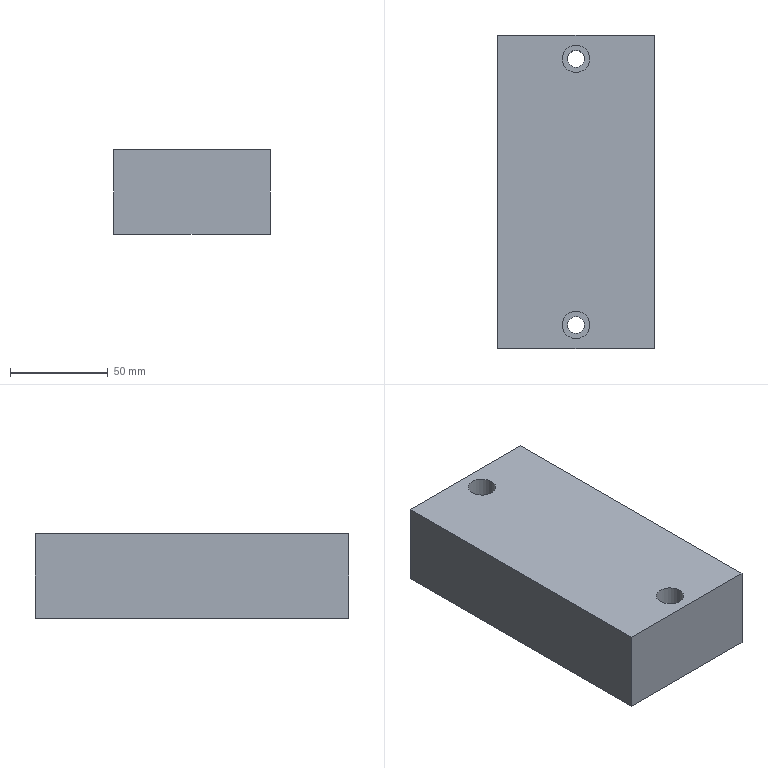Part | STEP file | 200 mesh_id2214 | 1 solid | 18 faces | box 80 x 160 x 43.2 mm | volume 542389 mm3 | plane 8 | cylinder 6 | cone 4 | commonest cylinder face diameters 6.8 x2 8.7 x2 14 x2
STEP:
#1=CARTESIAN_POINT('',(-16566.186,-4088.269,43.2));
#2=VERTEX_POINT('',#1);
#3=CARTESIAN_POINT('',(-16559.186,-4088.269,43.2));
#4=DIRECTION('',(0.,0.,-1.));
#5=DIRECTION('',(-1.,0.,0.));
#6=AXIS2_PLACEMENT_3D('',#3,#4,#5);
#7=CIRCLE('',#6,7.);
#8=EDGE_CURVE('',#2,#2,#7,.T.);
#9=ORIENTED_EDGE('',*,*,#8,.T.);
#10=EDGE_LOOP('',(#9));
#11=FACE_BOUND('',#10,.T.);
#12=CARTESIAN_POINT('',(-16566.186,-3952.269,43.2));
#13=VERTEX_POINT('',#12);
#14=CARTESIAN_POINT('',(-16559.186,-3952.269,43.2));
#15=DIRECTION('',(0.,0.,-1.));
#16=DIRECTION('',(-1.,0.,0.));
#17=AXIS2_PLACEMENT_3D('',#14,#15,#16);
#18=CIRCLE('',#17,7.);
#19=EDGE_CURVE('',#13,#13,#18,.T.);
#20=ORIENTED_EDGE('',*,*,#19,.T.);
#21=EDGE_LOOP('',(#20));
#22=FACE_BOUND('',#21,.T.);
#23=CARTESIAN_POINT('',(-16599.186,-3940.269,43.2));
#24=VERTEX_POINT('',#23);
#25=CARTESIAN_POINT('',(-16519.186,-3940.269,43.2));
#26=VERTEX_POINT('',#25);
#27=CARTESIAN_POINT('',(-16499.186,-3940.269,43.2));
#28=DIRECTION('',(1.,0.,0.));
#29=VECTOR('',#28,1.);
#30=LINE('',#27,#29);
#31=EDGE_CURVE('',#24,#26,#30,.T.);
#32=ORIENTED_EDGE('',*,*,#31,.F.);
#33=CARTESIAN_POINT('',(-16599.186,-4100.269,43.2));
#34=VERTEX_POINT('',#33);
#35=CARTESIAN_POINT('',(-16599.186,-3970.269,43.2));
#36=DIRECTION('',(0.,1.,0.));
#37=VECTOR('',#36,1.);
#38=LINE('',#35,#37);
#39=EDGE_CURVE('',#34,#24,#38,.T.);
#40=ORIENTED_EDGE('',*,*,#39,.F.);
#41=CARTESIAN_POINT('',(-16519.186,-4100.269,43.2));
#42=VERTEX_POINT('',#41);
#43=CARTESIAN_POINT('',(-16599.186,-4100.269,43.2));
#44=DIRECTION('',(-1.,0.,0.));
#45=VECTOR('',#44,1.);
#46=LINE('',#43,#45);
#47=EDGE_CURVE('',#42,#34,#46,.T.);
#48=ORIENTED_EDGE('',*,*,#47,.F.);
#49=CARTESIAN_POINT('',(-16519.186,-4070.269,43.2));
#50=DIRECTION('',(0.,-1.,0.));
#51=VECTOR('',#50,1.);
#52=LINE('',#49,#51);
#53=EDGE_CURVE('',#26,#42,#52,.T.);
#54=ORIENTED_EDGE('',*,*,#53,.F.);
#55=EDGE_LOOP('',(#32,#40,#48,#54));
#56=FACE_BOUND('',#55,.T.);
#57=CARTESIAN_POINT('',(-16648.884,-4140.769,43.2));
#58=DIRECTION('',(0.,0.,1.));
#59=DIRECTION('',(1.,0.,0.));
#60=AXIS2_PLACEMENT_3D('',#57,#58,#59);
#61=PLANE('',#60);
#62=ADVANCED_FACE('',(#11,#22,#56),#61,.T.);
#63=CARTESIAN_POINT('',(-16599.186,-4100.269,0.));
#64=VERTEX_POINT('',#63);
#65=CARTESIAN_POINT('',(-16599.186,-4100.269,0.));
#66=DIRECTION('',(0.,0.,1.));
#67=VECTOR('',#66,1.);
#68=LINE('',#65,#67);
#69=EDGE_CURVE('',#64,#34,#68,.T.);
#70=ORIENTED_EDGE('',*,*,#69,.T.);
#71=ORIENTED_EDGE('',*,*,#39,.T.);
#72=CARTESIAN_POINT('',(-16599.186,-3940.269,0.));
#73=VERTEX_POINT('',#72);
#74=CARTESIAN_POINT('',(-16599.186,-3940.269,0.));
#75=DIRECTION('',(0.,0.,1.));
#76=VECTOR('',#75,1.);
#77=LINE('',#74,#76);
#78=EDGE_CURVE('',#73,#24,#77,.T.);
#79=ORIENTED_EDGE('',*,*,#78,.F.);
#80=CARTESIAN_POINT('',(-16599.186,-3970.269,0.));
#81=DIRECTION('',(0.,-1.,0.));
#82=VECTOR('',#81,1.);
#83=LINE('',#80,#82);
#84=EDGE_CURVE('',#73,#64,#83,.T.);
#85=ORIENTED_EDGE('',*,*,#84,.T.);
#86=EDGE_LOOP('',(#70,#71,#79,#85));
#87=FACE_OUTER_BOUND('',#86,.T.);
#88=CARTESIAN_POINT('',(-16599.186,-3970.269,0.));
#89=DIRECTION('',(-1.,0.,0.));
#90=DIRECTION('',(0.,0.,1.));
#91=AXIS2_PLACEMENT_3D('',#88,#89,#90);
#92=PLANE('',#91);
#93=ADVANCED_FACE('',(#87),#92,.T.);
#94=CARTESIAN_POINT('',(-16554.836,-4088.269,0.));
#95=VERTEX_POINT('',#94);
#96=CARTESIAN_POINT('',(-16559.186,-4088.269,0.));
#97=DIRECTION('',(0.,0.,1.));
#98=DIRECTION('',(1.,0.,0.));
#99=AXIS2_PLACEMENT_3D('',#96,#97,#98);
#100=CIRCLE('',#99,4.35);
#101=EDGE_CURVE('',#95,#95,#100,.T.);
#102=ORIENTED_EDGE('',*,*,#101,.T.);
#103=EDGE_LOOP('',(#102));
#104=FACE_BOUND('',#103,.T.);
#105=CARTESIAN_POINT('',(-16554.836,-3952.269,0.));
#106=VERTEX_POINT('',#105);
#107=CARTESIAN_POINT('',(-16559.186,-3952.269,0.));
#108=DIRECTION('',(0.,0.,1.));
#109=DIRECTION('',(1.,0.,0.));
#110=AXIS2_PLACEMENT_3D('',#107,#108,#109);
#111=CIRCLE('',#110,4.35);
#112=EDGE_CURVE('',#106,#106,#111,.T.);
#113=ORIENTED_EDGE('',*,*,#112,.T.);
#114=EDGE_LOOP('',(#113));
#115=FACE_BOUND('',#114,.T.);
#116=CARTESIAN_POINT('',(-16583.186,-3952.269,0.));
#117=VERTEX_POINT('',#116);
#118=CARTESIAN_POINT('',(-16587.186,-3952.269,0.));
#119=DIRECTION('',(0.,0.,1.));
#120=DIRECTION('',(1.,0.,0.));
#121=AXIS2_PLACEMENT_3D('',#118,#119,#120);
#122=CIRCLE('',#121,4.);
#123=EDGE_CURVE('',#117,#117,#122,.T.);
#124=ORIENTED_EDGE('',*,*,#123,.T.);
#125=EDGE_LOOP('',(#124));
#126=FACE_BOUND('',#125,.T.);
#127=CARTESIAN_POINT('',(-16583.186,-4088.269,0.));
#128=VERTEX_POINT('',#127);
#129=CARTESIAN_POINT('',(-16587.186,-4088.269,0.));
#130=DIRECTION('',(0.,0.,1.));
#131=DIRECTION('',(1.,0.,0.));
#132=AXIS2_PLACEMENT_3D('',#129,#130,#131);
#133=CIRCLE('',#132,4.);
#134=EDGE_CURVE('',#128,#128,#133,.T.);
#135=ORIENTED_EDGE('',*,*,#134,.T.);
#136=EDGE_LOOP('',(#135));
#137=FACE_BOUND('',#136,.T.);
#138=CARTESIAN_POINT('',(-16519.186,-3940.269,0.));
#139=VERTEX_POINT('',#138);
#140=CARTESIAN_POINT('',(2.,-3940.269,0.));
#141=DIRECTION('',(-1.,0.,0.));
#142=VECTOR('',#141,1.);
#143=LINE('',#140,#142);
#144=EDGE_CURVE('',#139,#73,#143,.T.);
#145=ORIENTED_EDGE('',*,*,#144,.F.);
#146=CARTESIAN_POINT('',(-16519.186,-4100.269,0.));
#147=VERTEX_POINT('',#146);
#148=CARTESIAN_POINT('',(-16519.186,0.,0.));
#149=DIRECTION('',(0.,1.,0.));
#150=VECTOR('',#149,1.);
#151=LINE('',#148,#150);
#152=EDGE_CURVE('',#147,#139,#151,.T.);
#153=ORIENTED_EDGE('',*,*,#152,.F.);
#154=CARTESIAN_POINT('',(2.,-4100.269,0.));
#155=DIRECTION('',(1.,0.,0.));
#156=VECTOR('',#155,1.);
#157=LINE('',#154,#156);
#158=EDGE_CURVE('',#64,#147,#157,.T.);
#159=ORIENTED_EDGE('',*,*,#158,.F.);
#160=ORIENTED_EDGE('',*,*,#84,.F.);
#161=EDGE_LOOP('',(#145,#153,#159,#160));
#162=FACE_BOUND('',#161,.T.);
#163=CARTESIAN_POINT('',(2.,0.,0.));
#164=DIRECTION('',(0.,0.,1.));
#165=DIRECTION('',(1.,0.,0.));
#166=AXIS2_PLACEMENT_3D('',#163,#164,#165);
#167=PLANE('',#166);
#168=ADVANCED_FACE('',(#104,#115,#126,#137,#162),#167,.F.);
#169=CARTESIAN_POINT('',(-16519.186,-4100.269,0.));
#170=DIRECTION('',(0.,0.,1.));
#171=VECTOR('',#170,1.);
#172=LINE('',#169,#171);
#173=EDGE_CURVE('',#147,#42,#172,.T.);
#174=ORIENTED_EDGE('',*,*,#173,.T.);
#175=ORIENTED_EDGE('',*,*,#47,.T.);
#176=ORIENTED_EDGE('',*,*,#69,.F.);
#177=ORIENTED_EDGE('',*,*,#158,.T.);
#178=EDGE_LOOP('',(#174,#175,#176,#177));
#179=FACE_OUTER_BOUND('',#178,.T.);
#180=CARTESIAN_POINT('',(-16599.186,-4100.269,0.));
#181=DIRECTION('',(0.,-1.,0.));
#182=DIRECTION('',(0.,0.,-1.));
#183=AXIS2_PLACEMENT_3D('',#180,#181,#182);
#184=PLANE('',#183);
#185=ADVANCED_FACE('',(#179),#184,.T.);
#186=ORIENTED_EDGE('',*,*,#78,.T.);
#187=ORIENTED_EDGE('',*,*,#31,.T.);
#188=CARTESIAN_POINT('',(-16519.186,-3940.269,0.));
#189=DIRECTION('',(0.,0.,1.));
#190=VECTOR('',#189,1.);
#191=LINE('',#188,#190);
#192=EDGE_CURVE('',#139,#26,#191,.T.);
#193=ORIENTED_EDGE('',*,*,#192,.F.);
#194=ORIENTED_EDGE('',*,*,#144,.T.);
#195=EDGE_LOOP('',(#186,#187,#193,#194));
#196=FACE_OUTER_BOUND('',#195,.T.);
#197=CARTESIAN_POINT('',(-16499.186,-3940.269,0.));
#198=DIRECTION('',(0.,1.,0.));
#199=DIRECTION('',(0.,0.,1.));
#200=AXIS2_PLACEMENT_3D('',#197,#198,#199);
#201=PLANE('',#200);
#202=ADVANCED_FACE('',(#196),#201,.T.);
#203=ORIENTED_EDGE('',*,*,#192,.T.);
#204=ORIENTED_EDGE('',*,*,#53,.T.);
#205=ORIENTED_EDGE('',*,*,#173,.F.);
#206=ORIENTED_EDGE('',*,*,#152,.T.);
#207=EDGE_LOOP('',(#203,#204,#205,#206));
#208=FACE_OUTER_BOUND('',#207,.T.);
#209=CARTESIAN_POINT('',(-16519.186,-4070.269,0.));
#210=DIRECTION('',(1.,0.,0.));
#211=DIRECTION('',(0.,0.,-1.));
#212=AXIS2_PLACEMENT_3D('',#209,#210,#211);
#213=PLANE('',#212);
#214=ADVANCED_FACE('',(#208),#213,.T.);
#215=CARTESIAN_POINT('',(-16583.786,-4088.269,35.));
#216=VERTEX_POINT('',#215);
#217=CARTESIAN_POINT('',(-16587.186,-4088.269,35.));
#218=DIRECTION('',(0.,0.,-1.));
#219=DIRECTION('',(1.,0.,0.));
#220=AXIS2_PLACEMENT_3D('',#217,#218,#219);
#221=CIRCLE('',#220,3.4);
#222=EDGE_CURVE('',#216,#216,#221,.T.);
#223=ORIENTED_EDGE('',*,*,#222,.T.);
#224=EDGE_LOOP('',(#223));
#225=FACE_BOUND('',#224,.T.);
#226=CARTESIAN_POINT('',(-16587.186,-4088.269,37.043));
#227=VERTEX_POINT('',#226);
#228=VERTEX_LOOP('',#227);
#229=FACE_BOUND('',#228,.T.);
#230=CARTESIAN_POINT('',(-16587.186,-4088.269,35.));
#231=DIRECTION('',(0.,0.,-1.));
#232=DIRECTION('',(-1.,0.,0.));
#233=AXIS2_PLACEMENT_3D('',#230,#231,#232);
#234=CONICAL_SURFACE('',#233,3.4,59.);
#235=ADVANCED_FACE('',(#225,#229),#234,.F.);
#236=CARTESIAN_POINT('',(-16583.786,-4088.269,0.6));
#237=VERTEX_POINT('',#236);
#238=CARTESIAN_POINT('',(-16587.186,-4088.269,0.6));
#239=DIRECTION('',(0.,0.,-1.));
#240=DIRECTION('',(1.,0.,0.));
#241=AXIS2_PLACEMENT_3D('',#238,#239,#240);
#242=CIRCLE('',#241,3.4);
#243=EDGE_CURVE('',#237,#237,#242,.T.);
#244=ORIENTED_EDGE('',*,*,#243,.T.);
#245=EDGE_LOOP('',(#244));
#246=FACE_BOUND('',#245,.T.);
#247=ORIENTED_EDGE('',*,*,#222,.F.);
#248=EDGE_LOOP('',(#247));
#249=FACE_BOUND('',#248,.T.);
#250=CARTESIAN_POINT('',(-16587.186,-4088.269,0.));
#251=DIRECTION('',(0.,0.,1.));
#252=DIRECTION('',(1.,0.,0.));
#253=AXIS2_PLACEMENT_3D('',#250,#251,#252);
#254=CYLINDRICAL_SURFACE('',#253,3.4);
#255=ADVANCED_FACE('',(#246,#249),#254,.F.);
#256=ORIENTED_EDGE('',*,*,#243,.F.);
#257=EDGE_LOOP('',(#256));
#258=FACE_BOUND('',#257,.T.);
#259=ORIENTED_EDGE('',*,*,#134,.F.);
#260=EDGE_LOOP('',(#259));
#261=FACE_BOUND('',#260,.T.);
#262=CARTESIAN_POINT('',(-16587.186,-4088.269,0.));
#263=DIRECTION('',(0.,0.,-1.));
#264=DIRECTION('',(-1.,0.,0.));
#265=AXIS2_PLACEMENT_3D('',#262,#263,#264);
#266=CONICAL_SURFACE('',#265,4.,45.);
#267=ADVANCED_FACE('',(#258,#261),#266,.F.);
#268=CARTESIAN_POINT('',(-16583.786,-3952.269,35.));
#269=VERTEX_POINT('',#268);
#270=CARTESIAN_POINT('',(-16587.186,-3952.269,35.));
#271=DIRECTION('',(0.,0.,-1.));
#272=DIRECTION('',(1.,0.,0.));
#273=AXIS2_PLACEMENT_3D('',#270,#271,#272);
#274=CIRCLE('',#273,3.4);
#275=EDGE_CURVE('',#269,#269,#274,.T.);
#276=ORIENTED_EDGE('',*,*,#275,.T.);
#277=EDGE_LOOP('',(#276));
#278=FACE_BOUND('',#277,.T.);
#279=CARTESIAN_POINT('',(-16587.186,-3952.269,37.043));
#280=VERTEX_POINT('',#279);
#281=VERTEX_LOOP('',#280);
#282=FACE_BOUND('',#281,.T.);
#283=CARTESIAN_POINT('',(-16587.186,-3952.269,35.));
#284=DIRECTION('',(0.,0.,-1.));
#285=DIRECTION('',(-1.,0.,0.));
#286=AXIS2_PLACEMENT_3D('',#283,#284,#285);
#287=CONICAL_SURFACE('',#286,3.4,59.);
#288=ADVANCED_FACE('',(#278,#282),#287,.F.);
#289=CARTESIAN_POINT('',(-16583.786,-3952.269,0.6));
#290=VERTEX_POINT('',#289);
#291=CARTESIAN_POINT('',(-16587.186,-3952.269,0.6));
#292=DIRECTION('',(0.,0.,-1.));
#293=DIRECTION('',(1.,0.,0.));
#294=AXIS2_PLACEMENT_3D('',#291,#292,#293);
#295=CIRCLE('',#294,3.4);
#296=EDGE_CURVE('',#290,#290,#295,.T.);
#297=ORIENTED_EDGE('',*,*,#296,.T.);
#298=EDGE_LOOP('',(#297));
#299=FACE_BOUND('',#298,.T.);
#300=ORIENTED_EDGE('',*,*,#275,.F.);
#301=EDGE_LOOP('',(#300));
#302=FACE_BOUND('',#301,.T.);
#303=CARTESIAN_POINT('',(-16587.186,-3952.269,0.));
#304=DIRECTION('',(0.,0.,1.));
#305=DIRECTION('',(1.,0.,0.));
#306=AXIS2_PLACEMENT_3D('',#303,#304,#305);
#307=CYLINDRICAL_SURFACE('',#306,3.4);
#308=ADVANCED_FACE('',(#299,#302),#307,.F.);
#309=ORIENTED_EDGE('',*,*,#296,.F.);
#310=EDGE_LOOP('',(#309));
#311=FACE_BOUND('',#310,.T.);
#312=ORIENTED_EDGE('',*,*,#123,.F.);
#313=EDGE_LOOP('',(#312));
#314=FACE_BOUND('',#313,.T.);
#315=CARTESIAN_POINT('',(-16587.186,-3952.269,0.));
#316=DIRECTION('',(0.,0.,-1.));
#317=DIRECTION('',(-1.,0.,0.));
#318=AXIS2_PLACEMENT_3D('',#315,#316,#317);
#319=CONICAL_SURFACE('',#318,4.,45.);
#320=ADVANCED_FACE('',(#311,#314),#319,.F.);
#321=CARTESIAN_POINT('',(-16563.536,-3952.269,28.2));
#322=VERTEX_POINT('',#321);
#323=CARTESIAN_POINT('',(-16559.186,-3952.269,28.2));
#324=DIRECTION('',(0.,0.,1.));
#325=DIRECTION('',(-1.,0.,0.));
#326=AXIS2_PLACEMENT_3D('',#323,#324,#325);
#327=CIRCLE('',#326,4.35);
#328=EDGE_CURVE('',#322,#322,#327,.T.);
#329=ORIENTED_EDGE('',*,*,#328,.T.);
#330=EDGE_LOOP('',(#329));
#331=FACE_BOUND('',#330,.T.);
#332=ORIENTED_EDGE('',*,*,#112,.F.);
#333=EDGE_LOOP('',(#332));
#334=FACE_BOUND('',#333,.T.);
#335=CARTESIAN_POINT('',(-16559.186,-3952.269,-6.8));
#336=DIRECTION('',(0.,0.,-1.));
#337=DIRECTION('',(-1.,0.,0.));
#338=AXIS2_PLACEMENT_3D('',#335,#336,#337);
#339=CYLINDRICAL_SURFACE('',#338,4.35);
#340=ADVANCED_FACE('',(#331,#334),#339,.F.);
#341=ORIENTED_EDGE('',*,*,#328,.F.);
#342=EDGE_LOOP('',(#341));
#343=FACE_BOUND('',#342,.T.);
#344=CARTESIAN_POINT('',(-16566.186,-3952.269,28.2));
#345=VERTEX_POINT('',#344);
#346=CARTESIAN_POINT('',(-16559.186,-3952.269,28.2));
#347=DIRECTION('',(0.,0.,1.));
#348=DIRECTION('',(-1.,0.,0.));
#349=AXIS2_PLACEMENT_3D('',#346,#347,#348);
#350=CIRCLE('',#349,7.);
#351=EDGE_CURVE('',#345,#345,#350,.T.);
#352=ORIENTED_EDGE('',*,*,#351,.T.);
#353=EDGE_LOOP('',(#352));
#354=FACE_BOUND('',#353,.T.);
#355=CARTESIAN_POINT('',(-16559.186,-3952.269,28.2));
#356=DIRECTION('',(0.,0.,-1.));
#357=DIRECTION('',(-1.,0.,0.));
#358=AXIS2_PLACEMENT_3D('',#355,#356,#357);
#359=PLANE('',#358);
#360=ADVANCED_FACE('',(#343,#354),#359,.F.);
#361=ORIENTED_EDGE('',*,*,#351,.F.);
#362=EDGE_LOOP('',(#361));
#363=FACE_BOUND('',#362,.T.);
#364=ORIENTED_EDGE('',*,*,#19,.F.);
#365=EDGE_LOOP('',(#364));
#366=FACE_BOUND('',#365,.T.);
#367=CARTESIAN_POINT('',(-16559.186,-3952.269,43.2));
#368=DIRECTION('',(0.,0.,-1.));
#369=DIRECTION('',(-1.,0.,0.));
#370=AXIS2_PLACEMENT_3D('',#367,#368,#369);
#371=CYLINDRICAL_SURFACE('',#370,7.);
#372=ADVANCED_FACE('',(#363,#366),#371,.F.);
#373=CARTESIAN_POINT('',(-16563.536,-4088.269,28.2));
#374=VERTEX_POINT('',#373);
#375=CARTESIAN_POINT('',(-16559.186,-4088.269,28.2));
#376=DIRECTION('',(0.,0.,1.));
#377=DIRECTION('',(-1.,0.,0.));
#378=AXIS2_PLACEMENT_3D('',#375,#376,#377);
#379=CIRCLE('',#378,4.35);
#380=EDGE_CURVE('',#374,#374,#379,.T.);
#381=ORIENTED_EDGE('',*,*,#380,.T.);
#382=EDGE_LOOP('',(#381));
#383=FACE_BOUND('',#382,.T.);
#384=ORIENTED_EDGE('',*,*,#101,.F.);
#385=EDGE_LOOP('',(#384));
#386=FACE_BOUND('',#385,.T.);
#387=CARTESIAN_POINT('',(-16559.186,-4088.269,-6.8));
#388=DIRECTION('',(0.,0.,-1.));
#389=DIRECTION('',(-1.,0.,0.));
#390=AXIS2_PLACEMENT_3D('',#387,#388,#389);
#391=CYLINDRICAL_SURFACE('',#390,4.35);
#392=ADVANCED_FACE('',(#383,#386),#391,.F.);
#393=ORIENTED_EDGE('',*,*,#380,.F.);
#394=EDGE_LOOP('',(#393));
#395=FACE_BOUND('',#394,.T.);
#396=CARTESIAN_POINT('',(-16566.186,-4088.269,28.2));
#397=VERTEX_POINT('',#396);
#398=CARTESIAN_POINT('',(-16559.186,-4088.269,28.2));
#399=DIRECTION('',(0.,0.,1.));
#400=DIRECTION('',(-1.,0.,0.));
#401=AXIS2_PLACEMENT_3D('',#398,#399,#400);
#402=CIRCLE('',#401,7.);
#403=EDGE_CURVE('',#397,#397,#402,.T.);
#404=ORIENTED_EDGE('',*,*,#403,.T.);
#405=EDGE_LOOP('',(#404));
#406=FACE_BOUND('',#405,.T.);
#407=CARTESIAN_POINT('',(-16559.186,-4088.269,28.2));
#408=DIRECTION('',(0.,0.,-1.));
#409=DIRECTION('',(-1.,0.,0.));
#410=AXIS2_PLACEMENT_3D('',#407,#408,#409);
#411=PLANE('',#410);
#412=ADVANCED_FACE('',(#395,#406),#411,.F.);
#413=ORIENTED_EDGE('',*,*,#403,.F.);
#414=EDGE_LOOP('',(#413));
#415=FACE_BOUND('',#414,.T.);
#416=ORIENTED_EDGE('',*,*,#8,.F.);
#417=EDGE_LOOP('',(#416));
#418=FACE_BOUND('',#417,.T.);
#419=CARTESIAN_POINT('',(-16559.186,-4088.269,43.2));
#420=DIRECTION('',(0.,0.,-1.));
#421=DIRECTION('',(-1.,0.,0.));
#422=AXIS2_PLACEMENT_3D('',#419,#420,#421);
#423=CYLINDRICAL_SURFACE('',#422,7.);
#424=ADVANCED_FACE('',(#415,#418),#423,.F.);
#425=CLOSED_SHELL('',(#62,#93,#168,#185,#202,#214,#235,#255,#267,#288,#308,#320,#340,#360,#372,#392,#412,#424));
#426=MANIFOLD_SOLID_BREP('',#425);
#427=(LENGTH_UNIT()NAMED_UNIT(*)SI_UNIT(.MILLI.,.METRE.));
#428=UNCERTAINTY_MEASURE_WITH_UNIT(LENGTH_MEASURE(0.00002),#427,'','');
#429=(NAMED_UNIT(*)PLANE_ANGLE_UNIT()SI_UNIT($,.RADIAN.));
#430=PLANE_ANGLE_MEASURE_WITH_UNIT(PLANE_ANGLE_MEASURE(0.01745),#429);
#431=DIMENSIONAL_EXPONENTS(0.,0.,0.,0.,0.,0.,0.);
#432=(CONVERSION_BASED_UNIT('DEGREE',#430)NAMED_UNIT(#431)PLANE_ANGLE_UNIT());
#433=(NAMED_UNIT(*)SI_UNIT($,.STERADIAN.)SOLID_ANGLE_UNIT());
#434=(GEOMETRIC_REPRESENTATION_CONTEXT(3)GLOBAL_UNCERTAINTY_ASSIGNED_CONTEXT((#428))GLOBAL_UNIT_ASSIGNED_CONTEXT((#427,#432,#433))REPRESENTATION_CONTEXT('',''));
#435=ADVANCED_BREP_SHAPE_REPRESENTATION('',(#426),#434);